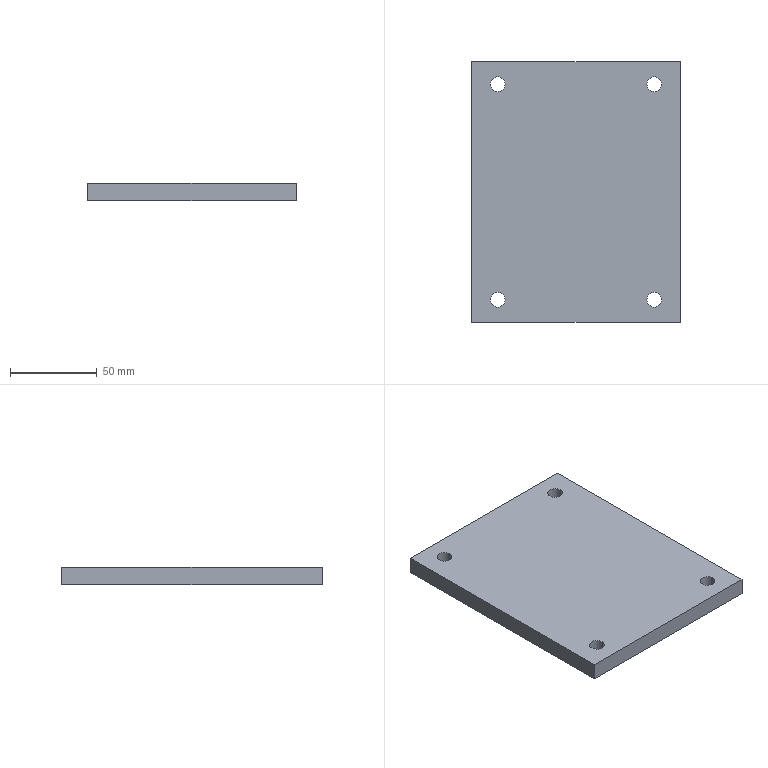Part | SolidWorks | features BaseBody 1 | 1 solid | 14 faces | box 120 x 150 x 10 mm | volume 177730 mm3 | cylinder 8 | plane 6 | commonest cylinder face diameters 8.5 x8
STEP:
#1=CARTESIAN_POINT('',(40.75,62.,-5.));
#2=VERTEX_POINT('',#1);
#3=CARTESIAN_POINT('',(49.25,62.,-5.));
#4=VERTEX_POINT('',#3);
#5=CARTESIAN_POINT('',(45.,62.,-5.));
#6=DIRECTION('',(0.,0.,1.));
#7=DIRECTION('',(1.,0.,0.));
#8=AXIS2_PLACEMENT_3D('',#5,#6,#7);
#9=CIRCLE('',#8,4.25);
#10=EDGE_CURVE('',#2,#4,#9,.T.);
#11=ORIENTED_EDGE('',*,*,#10,.F.);
#12=CARTESIAN_POINT('',(40.75,62.,5.));
#13=VERTEX_POINT('',#12);
#14=CARTESIAN_POINT('',(40.75,62.,-6.));
#15=DIRECTION('',(0.,0.,1.));
#16=VECTOR('',#15,1000.);
#17=LINE('',#14,#16);
#18=EDGE_CURVE('',#2,#13,#17,.T.);
#19=ORIENTED_EDGE('',*,*,#18,.T.);
#20=CARTESIAN_POINT('',(49.25,62.,5.));
#21=VERTEX_POINT('',#20);
#22=CARTESIAN_POINT('',(45.,62.,5.));
#23=DIRECTION('',(0.,0.,-1.));
#24=DIRECTION('',(1.,0.,0.));
#25=AXIS2_PLACEMENT_3D('',#22,#23,#24);
#26=CIRCLE('',#25,4.25);
#27=EDGE_CURVE('',#21,#13,#26,.T.);
#28=ORIENTED_EDGE('',*,*,#27,.F.);
#29=CARTESIAN_POINT('',(49.25,62.,-6.));
#30=DIRECTION('',(0.,0.,1.));
#31=VECTOR('',#30,1000.);
#32=LINE('',#29,#31);
#33=EDGE_CURVE('',#4,#21,#32,.T.);
#34=ORIENTED_EDGE('',*,*,#33,.F.);
#35=EDGE_LOOP('',(#11,#19,#28,#34));
#36=FACE_OUTER_BOUND('',#35,.T.);
#37=CARTESIAN_POINT('',(45.,62.,-6.));
#38=DIRECTION('',(0.,0.,1.));
#39=DIRECTION('',(1.,0.,0.));
#40=AXIS2_PLACEMENT_3D('',#37,#38,#39);
#41=CYLINDRICAL_SURFACE('',#40,4.25);
#42=ADVANCED_FACE('',(#36),#41,.F.);
#43=CARTESIAN_POINT('',(-49.25,62.,-5.));
#44=VERTEX_POINT('',#43);
#45=CARTESIAN_POINT('',(-40.75,62.,-5.));
#46=VERTEX_POINT('',#45);
#47=CARTESIAN_POINT('',(-45.,62.,-5.));
#48=DIRECTION('',(0.,0.,1.));
#49=DIRECTION('',(1.,0.,0.));
#50=AXIS2_PLACEMENT_3D('',#47,#48,#49);
#51=CIRCLE('',#50,4.25);
#52=EDGE_CURVE('',#44,#46,#51,.T.);
#53=ORIENTED_EDGE('',*,*,#52,.F.);
#54=CARTESIAN_POINT('',(-49.25,62.,5.));
#55=VERTEX_POINT('',#54);
#56=CARTESIAN_POINT('',(-49.25,62.,-6.));
#57=DIRECTION('',(0.,0.,1.));
#58=VECTOR('',#57,1000.);
#59=LINE('',#56,#58);
#60=EDGE_CURVE('',#44,#55,#59,.T.);
#61=ORIENTED_EDGE('',*,*,#60,.T.);
#62=CARTESIAN_POINT('',(-40.75,62.,5.));
#63=VERTEX_POINT('',#62);
#64=CARTESIAN_POINT('',(-45.,62.,5.));
#65=DIRECTION('',(0.,0.,-1.));
#66=DIRECTION('',(1.,0.,0.));
#67=AXIS2_PLACEMENT_3D('',#64,#65,#66);
#68=CIRCLE('',#67,4.25);
#69=EDGE_CURVE('',#63,#55,#68,.T.);
#70=ORIENTED_EDGE('',*,*,#69,.F.);
#71=CARTESIAN_POINT('',(-40.75,62.,-6.));
#72=DIRECTION('',(0.,0.,1.));
#73=VECTOR('',#72,1000.);
#74=LINE('',#71,#73);
#75=EDGE_CURVE('',#46,#63,#74,.T.);
#76=ORIENTED_EDGE('',*,*,#75,.F.);
#77=EDGE_LOOP('',(#53,#61,#70,#76));
#78=FACE_OUTER_BOUND('',#77,.T.);
#79=CARTESIAN_POINT('',(-45.,62.,-6.));
#80=DIRECTION('',(0.,0.,1.));
#81=DIRECTION('',(1.,0.,0.));
#82=AXIS2_PLACEMENT_3D('',#79,#80,#81);
#83=CYLINDRICAL_SURFACE('',#82,4.25);
#84=ADVANCED_FACE('',(#78),#83,.F.);
#85=CARTESIAN_POINT('',(40.75,-62.,-5.));
#86=VERTEX_POINT('',#85);
#87=CARTESIAN_POINT('',(49.25,-62.,-5.));
#88=VERTEX_POINT('',#87);
#89=CARTESIAN_POINT('',(45.,-62.,-5.));
#90=DIRECTION('',(0.,0.,1.));
#91=DIRECTION('',(1.,0.,0.));
#92=AXIS2_PLACEMENT_3D('',#89,#90,#91);
#93=CIRCLE('',#92,4.25);
#94=EDGE_CURVE('',#86,#88,#93,.T.);
#95=ORIENTED_EDGE('',*,*,#94,.F.);
#96=CARTESIAN_POINT('',(40.75,-62.,5.));
#97=VERTEX_POINT('',#96);
#98=CARTESIAN_POINT('',(40.75,-62.,-6.));
#99=DIRECTION('',(0.,0.,1.));
#100=VECTOR('',#99,1000.);
#101=LINE('',#98,#100);
#102=EDGE_CURVE('',#86,#97,#101,.T.);
#103=ORIENTED_EDGE('',*,*,#102,.T.);
#104=CARTESIAN_POINT('',(49.25,-62.,5.));
#105=VERTEX_POINT('',#104);
#106=CARTESIAN_POINT('',(45.,-62.,5.));
#107=DIRECTION('',(0.,0.,-1.));
#108=DIRECTION('',(1.,0.,0.));
#109=AXIS2_PLACEMENT_3D('',#106,#107,#108);
#110=CIRCLE('',#109,4.25);
#111=EDGE_CURVE('',#105,#97,#110,.T.);
#112=ORIENTED_EDGE('',*,*,#111,.F.);
#113=CARTESIAN_POINT('',(49.25,-62.,-6.));
#114=DIRECTION('',(0.,0.,1.));
#115=VECTOR('',#114,1000.);
#116=LINE('',#113,#115);
#117=EDGE_CURVE('',#88,#105,#116,.T.);
#118=ORIENTED_EDGE('',*,*,#117,.F.);
#119=EDGE_LOOP('',(#95,#103,#112,#118));
#120=FACE_OUTER_BOUND('',#119,.T.);
#121=CARTESIAN_POINT('',(45.,-62.,-6.));
#122=DIRECTION('',(0.,0.,1.));
#123=DIRECTION('',(1.,0.,0.));
#124=AXIS2_PLACEMENT_3D('',#121,#122,#123);
#125=CYLINDRICAL_SURFACE('',#124,4.25);
#126=ADVANCED_FACE('',(#120),#125,.F.);
#127=CARTESIAN_POINT('',(-49.25,-62.,-5.));
#128=VERTEX_POINT('',#127);
#129=CARTESIAN_POINT('',(-40.75,-62.,-5.));
#130=VERTEX_POINT('',#129);
#131=CARTESIAN_POINT('',(-45.,-62.,-5.));
#132=DIRECTION('',(0.,0.,1.));
#133=DIRECTION('',(1.,0.,0.));
#134=AXIS2_PLACEMENT_3D('',#131,#132,#133);
#135=CIRCLE('',#134,4.25);
#136=EDGE_CURVE('',#128,#130,#135,.T.);
#137=ORIENTED_EDGE('',*,*,#136,.F.);
#138=CARTESIAN_POINT('',(-49.25,-62.,5.));
#139=VERTEX_POINT('',#138);
#140=CARTESIAN_POINT('',(-49.25,-62.,-6.));
#141=DIRECTION('',(0.,0.,1.));
#142=VECTOR('',#141,1000.);
#143=LINE('',#140,#142);
#144=EDGE_CURVE('',#128,#139,#143,.T.);
#145=ORIENTED_EDGE('',*,*,#144,.T.);
#146=CARTESIAN_POINT('',(-40.75,-62.,5.));
#147=VERTEX_POINT('',#146);
#148=CARTESIAN_POINT('',(-45.,-62.,5.));
#149=DIRECTION('',(0.,0.,-1.));
#150=DIRECTION('',(1.,0.,0.));
#151=AXIS2_PLACEMENT_3D('',#148,#149,#150);
#152=CIRCLE('',#151,4.25);
#153=EDGE_CURVE('',#147,#139,#152,.T.);
#154=ORIENTED_EDGE('',*,*,#153,.F.);
#155=CARTESIAN_POINT('',(-40.75,-62.,-6.));
#156=DIRECTION('',(0.,0.,1.));
#157=VECTOR('',#156,1000.);
#158=LINE('',#155,#157);
#159=EDGE_CURVE('',#130,#147,#158,.T.);
#160=ORIENTED_EDGE('',*,*,#159,.F.);
#161=EDGE_LOOP('',(#137,#145,#154,#160));
#162=FACE_OUTER_BOUND('',#161,.T.);
#163=CARTESIAN_POINT('',(-45.,-62.,-6.));
#164=DIRECTION('',(0.,0.,1.));
#165=DIRECTION('',(1.,0.,0.));
#166=AXIS2_PLACEMENT_3D('',#163,#164,#165);
#167=CYLINDRICAL_SURFACE('',#166,4.25);
#168=ADVANCED_FACE('',(#162),#167,.F.);
#169=ORIENTED_EDGE('',*,*,#27,.T.);
#170=CARTESIAN_POINT('',(45.,62.,5.));
#171=DIRECTION('',(0.,0.,-1.));
#172=DIRECTION('',(1.,0.,0.));
#173=AXIS2_PLACEMENT_3D('',#170,#171,#172);
#174=CIRCLE('',#173,4.25);
#175=EDGE_CURVE('',#13,#21,#174,.T.);
#176=ORIENTED_EDGE('',*,*,#175,.T.);
#177=EDGE_LOOP('',(#169,#176));
#178=FACE_BOUND('',#177,.T.);
#179=ORIENTED_EDGE('',*,*,#69,.T.);
#180=CARTESIAN_POINT('',(-45.,62.,5.));
#181=DIRECTION('',(0.,0.,-1.));
#182=DIRECTION('',(1.,0.,0.));
#183=AXIS2_PLACEMENT_3D('',#180,#181,#182);
#184=CIRCLE('',#183,4.25);
#185=EDGE_CURVE('',#55,#63,#184,.T.);
#186=ORIENTED_EDGE('',*,*,#185,.T.);
#187=EDGE_LOOP('',(#179,#186));
#188=FACE_BOUND('',#187,.T.);
#189=ORIENTED_EDGE('',*,*,#111,.T.);
#190=CARTESIAN_POINT('',(45.,-62.,5.));
#191=DIRECTION('',(0.,0.,-1.));
#192=DIRECTION('',(1.,0.,0.));
#193=AXIS2_PLACEMENT_3D('',#190,#191,#192);
#194=CIRCLE('',#193,4.25);
#195=EDGE_CURVE('',#97,#105,#194,.T.);
#196=ORIENTED_EDGE('',*,*,#195,.T.);
#197=EDGE_LOOP('',(#189,#196));
#198=FACE_BOUND('',#197,.T.);
#199=ORIENTED_EDGE('',*,*,#153,.T.);
#200=CARTESIAN_POINT('',(-45.,-62.,5.));
#201=DIRECTION('',(0.,0.,-1.));
#202=DIRECTION('',(1.,0.,0.));
#203=AXIS2_PLACEMENT_3D('',#200,#201,#202);
#204=CIRCLE('',#203,4.25);
#205=EDGE_CURVE('',#139,#147,#204,.T.);
#206=ORIENTED_EDGE('',*,*,#205,.T.);
#207=EDGE_LOOP('',(#199,#206));
#208=FACE_BOUND('',#207,.T.);
#209=CARTESIAN_POINT('',(60.,-75.,5.));
#210=VERTEX_POINT('',#209);
#211=CARTESIAN_POINT('',(60.,75.,5.));
#212=VERTEX_POINT('',#211);
#213=CARTESIAN_POINT('',(60.,-75.,5.));
#214=DIRECTION('',(0.,1.,0.));
#215=VECTOR('',#214,1000.);
#216=LINE('',#213,#215);
#217=EDGE_CURVE('',#210,#212,#216,.T.);
#218=ORIENTED_EDGE('',*,*,#217,.T.);
#219=CARTESIAN_POINT('',(-60.,75.,5.));
#220=VERTEX_POINT('',#219);
#221=CARTESIAN_POINT('',(-60.,75.,5.));
#222=DIRECTION('',(-1.,0.,0.));
#223=VECTOR('',#222,1000.);
#224=LINE('',#221,#223);
#225=EDGE_CURVE('',#212,#220,#224,.T.);
#226=ORIENTED_EDGE('',*,*,#225,.T.);
#227=CARTESIAN_POINT('',(-60.,-75.,5.));
#228=VERTEX_POINT('',#227);
#229=CARTESIAN_POINT('',(-60.,-75.,5.));
#230=DIRECTION('',(0.,-1.,0.));
#231=VECTOR('',#230,1000.);
#232=LINE('',#229,#231);
#233=EDGE_CURVE('',#220,#228,#232,.T.);
#234=ORIENTED_EDGE('',*,*,#233,.T.);
#235=CARTESIAN_POINT('',(-60.,-75.,5.));
#236=DIRECTION('',(1.,0.,0.));
#237=VECTOR('',#236,1000.);
#238=LINE('',#235,#237);
#239=EDGE_CURVE('',#228,#210,#238,.T.);
#240=ORIENTED_EDGE('',*,*,#239,.T.);
#241=EDGE_LOOP('',(#218,#226,#234,#240));
#242=FACE_OUTER_BOUND('',#241,.T.);
#243=CARTESIAN_POINT('',(-60.,-75.,5.));
#244=DIRECTION('',(0.,0.,1.));
#245=DIRECTION('',(1.,0.,0.));
#246=AXIS2_PLACEMENT_3D('',#243,#244,#245);
#247=PLANE('',#246);
#248=ADVANCED_FACE('',(#178,#188,#198,#208,#242),#247,.T.);
#249=ORIENTED_EDGE('',*,*,#18,.F.);
#250=CARTESIAN_POINT('',(45.,62.,-5.));
#251=DIRECTION('',(0.,0.,1.));
#252=DIRECTION('',(1.,0.,0.));
#253=AXIS2_PLACEMENT_3D('',#250,#251,#252);
#254=CIRCLE('',#253,4.25);
#255=EDGE_CURVE('',#4,#2,#254,.T.);
#256=ORIENTED_EDGE('',*,*,#255,.F.);
#257=ORIENTED_EDGE('',*,*,#33,.T.);
#258=ORIENTED_EDGE('',*,*,#175,.F.);
#259=EDGE_LOOP('',(#249,#256,#257,#258));
#260=FACE_OUTER_BOUND('',#259,.T.);
#261=CARTESIAN_POINT('',(45.,62.,-6.));
#262=DIRECTION('',(0.,0.,1.));
#263=DIRECTION('',(1.,0.,0.));
#264=AXIS2_PLACEMENT_3D('',#261,#262,#263);
#265=CYLINDRICAL_SURFACE('',#264,4.25);
#266=ADVANCED_FACE('',(#260),#265,.F.);
#267=ORIENTED_EDGE('',*,*,#60,.F.);
#268=CARTESIAN_POINT('',(-45.,62.,-5.));
#269=DIRECTION('',(0.,0.,1.));
#270=DIRECTION('',(1.,0.,0.));
#271=AXIS2_PLACEMENT_3D('',#268,#269,#270);
#272=CIRCLE('',#271,4.25);
#273=EDGE_CURVE('',#46,#44,#272,.T.);
#274=ORIENTED_EDGE('',*,*,#273,.F.);
#275=ORIENTED_EDGE('',*,*,#75,.T.);
#276=ORIENTED_EDGE('',*,*,#185,.F.);
#277=EDGE_LOOP('',(#267,#274,#275,#276));
#278=FACE_OUTER_BOUND('',#277,.T.);
#279=CARTESIAN_POINT('',(-45.,62.,-6.));
#280=DIRECTION('',(0.,0.,1.));
#281=DIRECTION('',(1.,0.,0.));
#282=AXIS2_PLACEMENT_3D('',#279,#280,#281);
#283=CYLINDRICAL_SURFACE('',#282,4.25);
#284=ADVANCED_FACE('',(#278),#283,.F.);
#285=ORIENTED_EDGE('',*,*,#102,.F.);
#286=CARTESIAN_POINT('',(45.,-62.,-5.));
#287=DIRECTION('',(0.,0.,1.));
#288=DIRECTION('',(1.,0.,0.));
#289=AXIS2_PLACEMENT_3D('',#286,#287,#288);
#290=CIRCLE('',#289,4.25);
#291=EDGE_CURVE('',#88,#86,#290,.T.);
#292=ORIENTED_EDGE('',*,*,#291,.F.);
#293=ORIENTED_EDGE('',*,*,#117,.T.);
#294=ORIENTED_EDGE('',*,*,#195,.F.);
#295=EDGE_LOOP('',(#285,#292,#293,#294));
#296=FACE_OUTER_BOUND('',#295,.T.);
#297=CARTESIAN_POINT('',(45.,-62.,-6.));
#298=DIRECTION('',(0.,0.,1.));
#299=DIRECTION('',(1.,0.,0.));
#300=AXIS2_PLACEMENT_3D('',#297,#298,#299);
#301=CYLINDRICAL_SURFACE('',#300,4.25);
#302=ADVANCED_FACE('',(#296),#301,.F.);
#303=ORIENTED_EDGE('',*,*,#144,.F.);
#304=CARTESIAN_POINT('',(-45.,-62.,-5.));
#305=DIRECTION('',(0.,0.,1.));
#306=DIRECTION('',(1.,0.,0.));
#307=AXIS2_PLACEMENT_3D('',#304,#305,#306);
#308=CIRCLE('',#307,4.25);
#309=EDGE_CURVE('',#130,#128,#308,.T.);
#310=ORIENTED_EDGE('',*,*,#309,.F.);
#311=ORIENTED_EDGE('',*,*,#159,.T.);
#312=ORIENTED_EDGE('',*,*,#205,.F.);
#313=EDGE_LOOP('',(#303,#310,#311,#312));
#314=FACE_OUTER_BOUND('',#313,.T.);
#315=CARTESIAN_POINT('',(-45.,-62.,-6.));
#316=DIRECTION('',(0.,0.,1.));
#317=DIRECTION('',(1.,0.,0.));
#318=AXIS2_PLACEMENT_3D('',#315,#316,#317);
#319=CYLINDRICAL_SURFACE('',#318,4.25);
#320=ADVANCED_FACE('',(#314),#319,.F.);
#321=ORIENTED_EDGE('',*,*,#225,.F.);
#322=CARTESIAN_POINT('',(60.,75.,-5.));
#323=VERTEX_POINT('',#322);
#324=CARTESIAN_POINT('',(60.,75.,-5.));
#325=DIRECTION('',(0.,0.,-1.));
#326=VECTOR('',#325,1000.);
#327=LINE('',#324,#326);
#328=EDGE_CURVE('',#212,#323,#327,.T.);
#329=ORIENTED_EDGE('',*,*,#328,.T.);
#330=CARTESIAN_POINT('',(-60.,75.,-5.));
#331=VERTEX_POINT('',#330);
#332=CARTESIAN_POINT('',(-60.,75.,-5.));
#333=DIRECTION('',(-1.,0.,0.));
#334=VECTOR('',#333,1000.);
#335=LINE('',#332,#334);
#336=EDGE_CURVE('',#323,#331,#335,.T.);
#337=ORIENTED_EDGE('',*,*,#336,.T.);
#338=CARTESIAN_POINT('',(-60.,75.,-5.));
#339=DIRECTION('',(0.,0.,1.));
#340=VECTOR('',#339,1000.);
#341=LINE('',#338,#340);
#342=EDGE_CURVE('',#331,#220,#341,.T.);
#343=ORIENTED_EDGE('',*,*,#342,.T.);
#344=EDGE_LOOP('',(#321,#329,#337,#343));
#345=FACE_OUTER_BOUND('',#344,.T.);
#346=CARTESIAN_POINT('',(-60.,75.,-5.));
#347=DIRECTION('',(0.,1.,0.));
#348=DIRECTION('',(0.,0.,1.));
#349=AXIS2_PLACEMENT_3D('',#346,#347,#348);
#350=PLANE('',#349);
#351=ADVANCED_FACE('',(#345),#350,.T.);
#352=ORIENTED_EDGE('',*,*,#328,.F.);
#353=ORIENTED_EDGE('',*,*,#217,.F.);
#354=CARTESIAN_POINT('',(60.,-75.,-5.));
#355=VERTEX_POINT('',#354);
#356=CARTESIAN_POINT('',(60.,-75.,-5.));
#357=DIRECTION('',(0.,0.,-1.));
#358=VECTOR('',#357,1000.);
#359=LINE('',#356,#358);
#360=EDGE_CURVE('',#210,#355,#359,.T.);
#361=ORIENTED_EDGE('',*,*,#360,.T.);
#362=CARTESIAN_POINT('',(60.,-75.,-5.));
#363=DIRECTION('',(0.,1.,0.));
#364=VECTOR('',#363,1000.);
#365=LINE('',#362,#364);
#366=EDGE_CURVE('',#355,#323,#365,.T.);
#367=ORIENTED_EDGE('',*,*,#366,.T.);
#368=EDGE_LOOP('',(#352,#353,#361,#367));
#369=FACE_OUTER_BOUND('',#368,.T.);
#370=CARTESIAN_POINT('',(60.,-75.,-5.));
#371=DIRECTION('',(1.,0.,0.));
#372=DIRECTION('',(0.,0.,-1.));
#373=AXIS2_PLACEMENT_3D('',#370,#371,#372);
#374=PLANE('',#373);
#375=ADVANCED_FACE('',(#369),#374,.T.);
#376=ORIENTED_EDGE('',*,*,#239,.F.);
#377=CARTESIAN_POINT('',(-60.,-75.,-5.));
#378=VERTEX_POINT('',#377);
#379=CARTESIAN_POINT('',(-60.,-75.,-5.));
#380=DIRECTION('',(0.,0.,1.));
#381=VECTOR('',#380,1000.);
#382=LINE('',#379,#381);
#383=EDGE_CURVE('',#378,#228,#382,.T.);
#384=ORIENTED_EDGE('',*,*,#383,.F.);
#385=CARTESIAN_POINT('',(-60.,-75.,-5.));
#386=DIRECTION('',(-1.,0.,0.));
#387=VECTOR('',#386,1000.);
#388=LINE('',#385,#387);
#389=EDGE_CURVE('',#355,#378,#388,.T.);
#390=ORIENTED_EDGE('',*,*,#389,.F.);
#391=ORIENTED_EDGE('',*,*,#360,.F.);
#392=EDGE_LOOP('',(#376,#384,#390,#391));
#393=FACE_OUTER_BOUND('',#392,.T.);
#394=CARTESIAN_POINT('',(-60.,-75.,-5.));
#395=DIRECTION('',(0.,1.,0.));
#396=DIRECTION('',(0.,0.,1.));
#397=AXIS2_PLACEMENT_3D('',#394,#395,#396);
#398=PLANE('',#397);
#399=ADVANCED_FACE('',(#393),#398,.F.);
#400=ORIENTED_EDGE('',*,*,#342,.F.);
#401=CARTESIAN_POINT('',(-60.,-75.,-5.));
#402=DIRECTION('',(0.,1.,0.));
#403=VECTOR('',#402,1000.);
#404=LINE('',#401,#403);
#405=EDGE_CURVE('',#378,#331,#404,.T.);
#406=ORIENTED_EDGE('',*,*,#405,.F.);
#407=ORIENTED_EDGE('',*,*,#383,.T.);
#408=ORIENTED_EDGE('',*,*,#233,.F.);
#409=EDGE_LOOP('',(#400,#406,#407,#408));
#410=FACE_OUTER_BOUND('',#409,.T.);
#411=CARTESIAN_POINT('',(-60.,-75.,-5.));
#412=DIRECTION('',(1.,0.,0.));
#413=DIRECTION('',(0.,0.,-1.));
#414=AXIS2_PLACEMENT_3D('',#411,#412,#413);
#415=PLANE('',#414);
#416=ADVANCED_FACE('',(#410),#415,.F.);
#417=ORIENTED_EDGE('',*,*,#255,.T.);
#418=ORIENTED_EDGE('',*,*,#10,.T.);
#419=EDGE_LOOP('',(#417,#418));
#420=FACE_BOUND('',#419,.T.);
#421=ORIENTED_EDGE('',*,*,#273,.T.);
#422=ORIENTED_EDGE('',*,*,#52,.T.);
#423=EDGE_LOOP('',(#421,#422));
#424=FACE_BOUND('',#423,.T.);
#425=ORIENTED_EDGE('',*,*,#291,.T.);
#426=ORIENTED_EDGE('',*,*,#94,.T.);
#427=EDGE_LOOP('',(#425,#426));
#428=FACE_BOUND('',#427,.T.);
#429=ORIENTED_EDGE('',*,*,#309,.T.);
#430=ORIENTED_EDGE('',*,*,#136,.T.);
#431=EDGE_LOOP('',(#429,#430));
#432=FACE_BOUND('',#431,.T.);
#433=ORIENTED_EDGE('',*,*,#366,.F.);
#434=ORIENTED_EDGE('',*,*,#389,.T.);
#435=ORIENTED_EDGE('',*,*,#405,.T.);
#436=ORIENTED_EDGE('',*,*,#336,.F.);
#437=EDGE_LOOP('',(#433,#434,#435,#436));
#438=FACE_OUTER_BOUND('',#437,.T.);
#439=CARTESIAN_POINT('',(-60.,-75.,-5.));
#440=DIRECTION('',(0.,0.,1.));
#441=DIRECTION('',(1.,0.,0.));
#442=AXIS2_PLACEMENT_3D('',#439,#440,#441);
#443=PLANE('',#442);
#444=ADVANCED_FACE('',(#420,#424,#428,#432,#438),#443,.F.);
#445=CLOSED_SHELL('',(#42,#84,#126,#168,#248,#266,#284,#302,#320,#351,#375,#399,#416,#444));
#446=MANIFOLD_SOLID_BREP('',#445);
#447=CARTESIAN_POINT('',(0.,0.,0.));
#448=DIRECTION('',(0.,0.,1.));
#449=DIRECTION('',(1.,0.,0.));
#450=AXIS2_PLACEMENT_3D('',#447,#448,#449);
#451=(LENGTH_UNIT()NAMED_UNIT(*)SI_UNIT(.MILLI.,.METRE.));
#452=UNCERTAINTY_MEASURE_WITH_UNIT(LENGTH_MEASURE(0.00001),#451,'','');
#453=(NAMED_UNIT(*)PLANE_ANGLE_UNIT()SI_UNIT($,.RADIAN.));
#454=(NAMED_UNIT(*)SI_UNIT($,.STERADIAN.)SOLID_ANGLE_UNIT());
#455=(GEOMETRIC_REPRESENTATION_CONTEXT(3)GLOBAL_UNCERTAINTY_ASSIGNED_CONTEXT((#452))GLOBAL_UNIT_ASSIGNED_CONTEXT((#451,#453,#454))REPRESENTATION_CONTEXT('',''));
#456=ADVANCED_BREP_SHAPE_REPRESENTATION('',(#446,#450),#455);